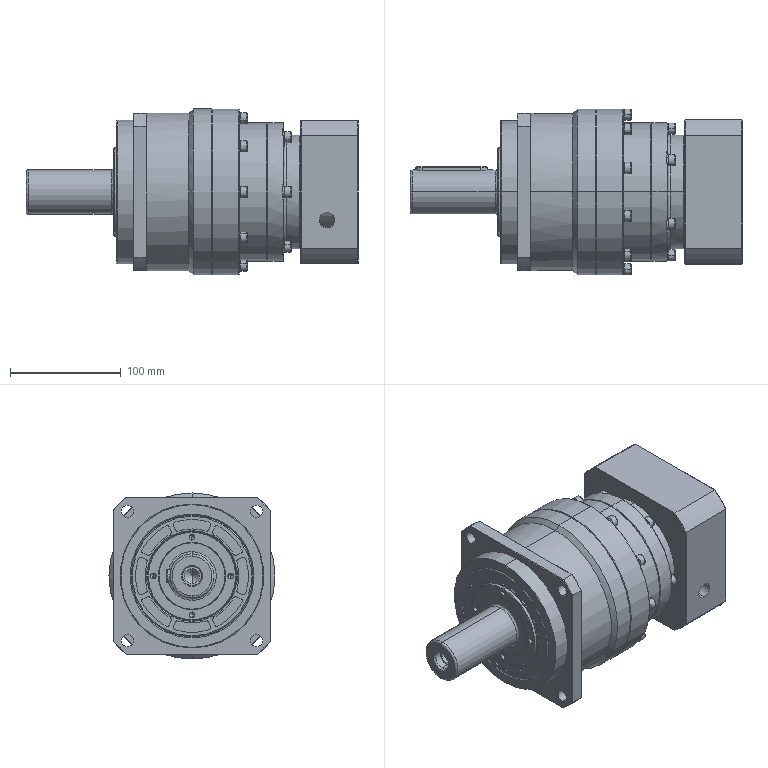Part | SolidWorks | features BaseBody 51 | 51 solids | 1322 faces | box 300 x 150 x 150 mm | volume 3045756 mm3 | plane 581 | cylinder 468 | cone 223 | spline 50 | commonest cylinder face diameters 6.68 x66 9.88 x66 6 x44 6.6 x44 10 x44 4 x40